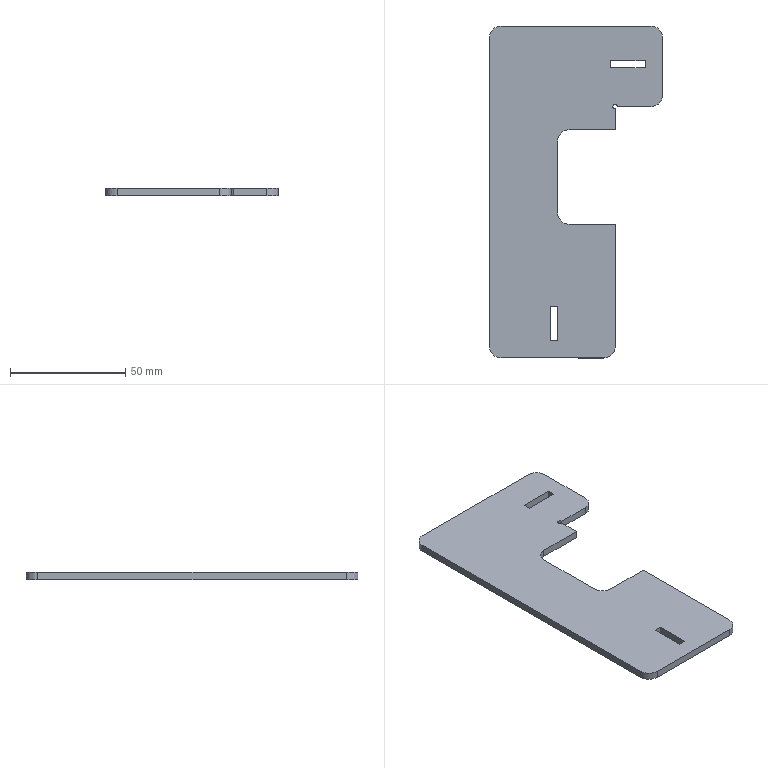Part | SolidWorks | features FlatPattern 1, SMBaseFlange 1, SheetMetal 1 | 1 solid | 29 faces | box 75 x 144 x 3.2 mm | volume 23763 mm3 | plane 20 | cylinder 9 | commonest cylinder face diameters 10 x7 2 x2
STEP:
#1=CARTESIAN_POINT('',(-21.5,109.,3.2));
#2=VERTEX_POINT('',#1);
#3=CARTESIAN_POINT('',(-19.5,109.,3.2));
#4=VERTEX_POINT('',#3);
#5=CARTESIAN_POINT('',(-20.5,109.,3.2));
#6=DIRECTION('',(0.,0.,-1.));
#7=DIRECTION('',(1.,0.,0.));
#8=AXIS2_PLACEMENT_3D('',#5,#6,#7);
#9=CIRCLE('',#8,1.);
#10=EDGE_CURVE('',#2,#4,#9,.T.);
#11=ORIENTED_EDGE('',*,*,#10,.F.);
#12=CARTESIAN_POINT('',(-21.5,109.,0.));
#13=VERTEX_POINT('',#12);
#14=CARTESIAN_POINT('',(-21.5,109.,3.2));
#15=DIRECTION('',(0.,0.,-1.));
#16=VECTOR('',#15,1000.);
#17=LINE('',#14,#16);
#18=EDGE_CURVE('',#2,#13,#17,.T.);
#19=ORIENTED_EDGE('',*,*,#18,.T.);
#20=CARTESIAN_POINT('',(-19.5,109.,0.));
#21=VERTEX_POINT('',#20);
#22=CARTESIAN_POINT('',(-20.5,109.,0.));
#23=DIRECTION('',(0.,0.,-1.));
#24=DIRECTION('',(1.,0.,0.));
#25=AXIS2_PLACEMENT_3D('',#22,#23,#24);
#26=CIRCLE('',#25,1.);
#27=EDGE_CURVE('',#13,#21,#26,.T.);
#28=ORIENTED_EDGE('',*,*,#27,.T.);
#29=CARTESIAN_POINT('',(-19.5,109.,3.2));
#30=DIRECTION('',(0.,0.,-1.));
#31=VECTOR('',#30,1000.);
#32=LINE('',#29,#31);
#33=EDGE_CURVE('',#4,#21,#32,.T.);
#34=ORIENTED_EDGE('',*,*,#33,.F.);
#35=EDGE_LOOP('',(#11,#19,#28,#34));
#36=FACE_OUTER_BOUND('',#35,.T.);
#37=CARTESIAN_POINT('',(-20.5,109.,3.2));
#38=DIRECTION('',(0.,0.,-1.));
#39=DIRECTION('',(-1.,0.,0.));
#40=AXIS2_PLACEMENT_3D('',#37,#38,#39);
#41=CYLINDRICAL_SURFACE('',#40,1.);
#42=ADVANCED_FACE('',(#36),#41,.F.);
#43=CARTESIAN_POINT('',(-7.5,125.8,3.2));
#44=VERTEX_POINT('',#43);
#45=CARTESIAN_POINT('',(-7.5,129.,3.2));
#46=VERTEX_POINT('',#45);
#47=CARTESIAN_POINT('',(-7.5,129.,3.2));
#48=DIRECTION('',(0.,1.,0.));
#49=VECTOR('',#48,1000.);
#50=LINE('',#47,#49);
#51=EDGE_CURVE('',#44,#46,#50,.T.);
#52=ORIENTED_EDGE('',*,*,#51,.F.);
#53=CARTESIAN_POINT('',(-22.5,125.8,3.2));
#54=VERTEX_POINT('',#53);
#55=CARTESIAN_POINT('',(-7.5,125.8,3.2));
#56=DIRECTION('',(1.,0.,0.));
#57=VECTOR('',#56,1000.);
#58=LINE('',#55,#57);
#59=EDGE_CURVE('',#54,#44,#58,.T.);
#60=ORIENTED_EDGE('',*,*,#59,.F.);
#61=CARTESIAN_POINT('',(-22.5,129.,3.2));
#62=VERTEX_POINT('',#61);
#63=CARTESIAN_POINT('',(-22.5,129.,3.2));
#64=DIRECTION('',(0.,-1.,0.));
#65=VECTOR('',#64,1000.);
#66=LINE('',#63,#65);
#67=EDGE_CURVE('',#62,#54,#66,.T.);
#68=ORIENTED_EDGE('',*,*,#67,.F.);
#69=CARTESIAN_POINT('',(-7.5,129.,3.2));
#70=DIRECTION('',(-1.,0.,0.));
#71=VECTOR('',#70,1000.);
#72=LINE('',#69,#71);
#73=EDGE_CURVE('',#46,#62,#72,.T.);
#74=ORIENTED_EDGE('',*,*,#73,.F.);
#75=EDGE_LOOP('',(#52,#60,#68,#74));
#76=FACE_BOUND('',#75,.T.);
#77=CARTESIAN_POINT('',(-40.5,58.,3.2));
#78=VERTEX_POINT('',#77);
#79=CARTESIAN_POINT('',(-45.5,63.,3.2));
#80=VERTEX_POINT('',#79);
#81=CARTESIAN_POINT('',(-40.5,63.,3.2));
#82=DIRECTION('',(0.,0.,-1.));
#83=DIRECTION('',(-1.,0.,0.));
#84=AXIS2_PLACEMENT_3D('',#81,#82,#83);
#85=CIRCLE('',#84,5.);
#86=EDGE_CURVE('',#78,#80,#85,.T.);
#87=ORIENTED_EDGE('',*,*,#86,.T.);
#88=CARTESIAN_POINT('',(-45.5,94.,3.2));
#89=VERTEX_POINT('',#88);
#90=CARTESIAN_POINT('',(-45.5,63.,3.2));
#91=DIRECTION('',(0.,1.,0.));
#92=VECTOR('',#91,1000.);
#93=LINE('',#90,#92);
#94=EDGE_CURVE('',#80,#89,#93,.T.);
#95=ORIENTED_EDGE('',*,*,#94,.T.);
#96=CARTESIAN_POINT('',(-40.5,99.,3.2));
#97=VERTEX_POINT('',#96);
#98=CARTESIAN_POINT('',(-40.5,94.,3.2));
#99=DIRECTION('',(0.,0.,-1.));
#100=DIRECTION('',(-1.,0.,0.));
#101=AXIS2_PLACEMENT_3D('',#98,#99,#100);
#102=CIRCLE('',#101,5.);
#103=EDGE_CURVE('',#89,#97,#102,.T.);
#104=ORIENTED_EDGE('',*,*,#103,.T.);
#105=CARTESIAN_POINT('',(-20.5,99.,3.2));
#106=VERTEX_POINT('',#105);
#107=CARTESIAN_POINT('',(-40.5,99.,3.2));
#108=DIRECTION('',(1.,0.,0.));
#109=VECTOR('',#108,1000.);
#110=LINE('',#107,#109);
#111=EDGE_CURVE('',#97,#106,#110,.T.);
#112=ORIENTED_EDGE('',*,*,#111,.T.);
#113=CARTESIAN_POINT('',(-20.5,108.,3.2));
#114=VERTEX_POINT('',#113);
#115=CARTESIAN_POINT('',(-20.5,99.,3.2));
#116=DIRECTION('',(0.,1.,0.));
#117=VECTOR('',#116,1000.);
#118=LINE('',#115,#117);
#119=EDGE_CURVE('',#106,#114,#118,.T.);
#120=ORIENTED_EDGE('',*,*,#119,.T.);
#121=CARTESIAN_POINT('',(-20.5,109.,3.2));
#122=DIRECTION('',(0.,0.,-1.));
#123=DIRECTION('',(1.,0.,0.));
#124=AXIS2_PLACEMENT_3D('',#121,#122,#123);
#125=CIRCLE('',#124,1.);
#126=EDGE_CURVE('',#114,#2,#125,.T.);
#127=ORIENTED_EDGE('',*,*,#126,.T.);
#128=ORIENTED_EDGE('',*,*,#10,.T.);
#129=CARTESIAN_POINT('',(-5.,109.,3.2));
#130=VERTEX_POINT('',#129);
#131=CARTESIAN_POINT('',(-19.5,109.,3.2));
#132=DIRECTION('',(1.,0.,0.));
#133=VECTOR('',#132,1000.);
#134=LINE('',#131,#133);
#135=EDGE_CURVE('',#4,#130,#134,.T.);
#136=ORIENTED_EDGE('',*,*,#135,.T.);
#137=CARTESIAN_POINT('',(0.,114.,3.2));
#138=VERTEX_POINT('',#137);
#139=CARTESIAN_POINT('',(-5.,114.,3.2));
#140=DIRECTION('',(0.,0.,1.));
#141=DIRECTION('',(1.,0.,0.));
#142=AXIS2_PLACEMENT_3D('',#139,#140,#141);
#143=CIRCLE('',#142,5.);
#144=EDGE_CURVE('',#130,#138,#143,.T.);
#145=ORIENTED_EDGE('',*,*,#144,.T.);
#146=CARTESIAN_POINT('',(0.,139.,3.2));
#147=VERTEX_POINT('',#146);
#148=CARTESIAN_POINT('',(0.,114.,3.2));
#149=DIRECTION('',(0.,1.,0.));
#150=VECTOR('',#149,1000.);
#151=LINE('',#148,#150);
#152=EDGE_CURVE('',#138,#147,#151,.T.);
#153=ORIENTED_EDGE('',*,*,#152,.T.);
#154=CARTESIAN_POINT('',(-5.,144.,3.2));
#155=VERTEX_POINT('',#154);
#156=CARTESIAN_POINT('',(-5.,139.,3.2));
#157=DIRECTION('',(0.,0.,1.));
#158=DIRECTION('',(-1.,0.,0.));
#159=AXIS2_PLACEMENT_3D('',#156,#157,#158);
#160=CIRCLE('',#159,5.);
#161=EDGE_CURVE('',#147,#155,#160,.T.);
#162=ORIENTED_EDGE('',*,*,#161,.T.);
#163=CARTESIAN_POINT('',(-70.,144.,3.2));
#164=VERTEX_POINT('',#163);
#165=CARTESIAN_POINT('',(-5.,144.,3.2));
#166=DIRECTION('',(-1.,0.,0.));
#167=VECTOR('',#166,1000.);
#168=LINE('',#165,#167);
#169=EDGE_CURVE('',#155,#164,#168,.T.);
#170=ORIENTED_EDGE('',*,*,#169,.T.);
#171=CARTESIAN_POINT('',(-75.,139.,3.2));
#172=VERTEX_POINT('',#171);
#173=CARTESIAN_POINT('',(-70.,139.,3.2));
#174=DIRECTION('',(0.,0.,1.));
#175=DIRECTION('',(1.,0.,0.));
#176=AXIS2_PLACEMENT_3D('',#173,#174,#175);
#177=CIRCLE('',#176,5.);
#178=EDGE_CURVE('',#164,#172,#177,.T.);
#179=ORIENTED_EDGE('',*,*,#178,.T.);
#180=CARTESIAN_POINT('',(-75.,5.,3.2));
#181=VERTEX_POINT('',#180);
#182=CARTESIAN_POINT('',(-75.,139.,3.2));
#183=DIRECTION('',(0.,-1.,0.));
#184=VECTOR('',#183,1000.);
#185=LINE('',#182,#184);
#186=EDGE_CURVE('',#172,#181,#185,.T.);
#187=ORIENTED_EDGE('',*,*,#186,.T.);
#188=CARTESIAN_POINT('',(-70.,0.,3.2));
#189=VERTEX_POINT('',#188);
#190=CARTESIAN_POINT('',(-70.,5.,3.2));
#191=DIRECTION('',(0.,0.,1.));
#192=DIRECTION('',(1.,0.,0.));
#193=AXIS2_PLACEMENT_3D('',#190,#191,#192);
#194=CIRCLE('',#193,5.);
#195=EDGE_CURVE('',#181,#189,#194,.T.);
#196=ORIENTED_EDGE('',*,*,#195,.T.);
#197=CARTESIAN_POINT('',(-25.5,0.,3.2));
#198=VERTEX_POINT('',#197);
#199=CARTESIAN_POINT('',(-25.5,0.,3.2));
#200=DIRECTION('',(1.,0.,0.));
#201=VECTOR('',#200,1000.);
#202=LINE('',#199,#201);
#203=EDGE_CURVE('',#189,#198,#202,.T.);
#204=ORIENTED_EDGE('',*,*,#203,.T.);
#205=CARTESIAN_POINT('',(-20.5,5.,3.2));
#206=VERTEX_POINT('',#205);
#207=CARTESIAN_POINT('',(-25.5,5.,3.2));
#208=DIRECTION('',(0.,0.,1.));
#209=DIRECTION('',(-1.,0.,0.));
#210=AXIS2_PLACEMENT_3D('',#207,#208,#209);
#211=CIRCLE('',#210,5.);
#212=EDGE_CURVE('',#198,#206,#211,.T.);
#213=ORIENTED_EDGE('',*,*,#212,.T.);
#214=CARTESIAN_POINT('',(-20.5,58.,3.2));
#215=VERTEX_POINT('',#214);
#216=CARTESIAN_POINT('',(-20.5,58.,3.2));
#217=DIRECTION('',(0.,1.,0.));
#218=VECTOR('',#217,1000.);
#219=LINE('',#216,#218);
#220=EDGE_CURVE('',#206,#215,#219,.T.);
#221=ORIENTED_EDGE('',*,*,#220,.T.);
#222=CARTESIAN_POINT('',(-20.5,58.,3.2));
#223=DIRECTION('',(-1.,0.,0.));
#224=VECTOR('',#223,1000.);
#225=LINE('',#222,#224);
#226=EDGE_CURVE('',#215,#78,#225,.T.);
#227=ORIENTED_EDGE('',*,*,#226,.T.);
#228=EDGE_LOOP('',(#87,#95,#104,#112,#120,#127,#128,#136,#145,#153,#162,#170,#179,#187,#196,#204,#213,#221,#227));
#229=FACE_OUTER_BOUND('',#228,.T.);
#230=CARTESIAN_POINT('',(-45.5,7.5,3.2));
#231=VERTEX_POINT('',#230);
#232=CARTESIAN_POINT('',(-45.5,22.5,3.2));
#233=VERTEX_POINT('',#232);
#234=CARTESIAN_POINT('',(-45.5,7.5,3.2));
#235=DIRECTION('',(0.,1.,0.));
#236=VECTOR('',#235,1000.);
#237=LINE('',#234,#236);
#238=EDGE_CURVE('',#231,#233,#237,.T.);
#239=ORIENTED_EDGE('',*,*,#238,.F.);
#240=CARTESIAN_POINT('',(-48.7,7.5,3.2));
#241=VERTEX_POINT('',#240);
#242=CARTESIAN_POINT('',(-45.5,7.5,3.2));
#243=DIRECTION('',(1.,0.,0.));
#244=VECTOR('',#243,1000.);
#245=LINE('',#242,#244);
#246=EDGE_CURVE('',#241,#231,#245,.T.);
#247=ORIENTED_EDGE('',*,*,#246,.F.);
#248=CARTESIAN_POINT('',(-48.7,22.5,3.2));
#249=VERTEX_POINT('',#248);
#250=CARTESIAN_POINT('',(-48.7,7.5,3.2));
#251=DIRECTION('',(0.,-1.,0.));
#252=VECTOR('',#251,1000.);
#253=LINE('',#250,#252);
#254=EDGE_CURVE('',#249,#241,#253,.T.);
#255=ORIENTED_EDGE('',*,*,#254,.F.);
#256=CARTESIAN_POINT('',(-45.5,22.5,3.2));
#257=DIRECTION('',(-1.,0.,0.));
#258=VECTOR('',#257,1000.);
#259=LINE('',#256,#258);
#260=EDGE_CURVE('',#233,#249,#259,.T.);
#261=ORIENTED_EDGE('',*,*,#260,.F.);
#262=EDGE_LOOP('',(#239,#247,#255,#261));
#263=FACE_BOUND('',#262,.T.);
#264=CARTESIAN_POINT('',(-40.5,63.,3.2));
#265=DIRECTION('',(0.,0.,-1.));
#266=DIRECTION('',(-1.,0.,0.));
#267=AXIS2_PLACEMENT_3D('',#264,#265,#266);
#268=PLANE('',#267);
#269=ADVANCED_FACE('',(#76,#229,#263),#268,.F.);
#270=CARTESIAN_POINT('',(-40.5,58.,0.));
#271=VERTEX_POINT('',#270);
#272=CARTESIAN_POINT('',(-45.5,63.,0.));
#273=VERTEX_POINT('',#272);
#274=CARTESIAN_POINT('',(-40.5,63.,0.));
#275=DIRECTION('',(0.,0.,-1.));
#276=DIRECTION('',(-1.,0.,0.));
#277=AXIS2_PLACEMENT_3D('',#274,#275,#276);
#278=CIRCLE('',#277,5.);
#279=EDGE_CURVE('',#271,#273,#278,.T.);
#280=ORIENTED_EDGE('',*,*,#279,.F.);
#281=CARTESIAN_POINT('',(-20.5,58.,0.));
#282=VERTEX_POINT('',#281);
#283=CARTESIAN_POINT('',(-20.5,58.,0.));
#284=DIRECTION('',(-1.,0.,0.));
#285=VECTOR('',#284,1000.);
#286=LINE('',#283,#285);
#287=EDGE_CURVE('',#282,#271,#286,.T.);
#288=ORIENTED_EDGE('',*,*,#287,.F.);
#289=CARTESIAN_POINT('',(-20.5,5.,0.));
#290=VERTEX_POINT('',#289);
#291=CARTESIAN_POINT('',(-20.5,58.,0.));
#292=DIRECTION('',(0.,1.,0.));
#293=VECTOR('',#292,1000.);
#294=LINE('',#291,#293);
#295=EDGE_CURVE('',#290,#282,#294,.T.);
#296=ORIENTED_EDGE('',*,*,#295,.F.);
#297=CARTESIAN_POINT('',(-25.5,0.,0.));
#298=VERTEX_POINT('',#297);
#299=CARTESIAN_POINT('',(-25.5,5.,0.));
#300=DIRECTION('',(0.,0.,1.));
#301=DIRECTION('',(-1.,0.,0.));
#302=AXIS2_PLACEMENT_3D('',#299,#300,#301);
#303=CIRCLE('',#302,5.);
#304=EDGE_CURVE('',#298,#290,#303,.T.);
#305=ORIENTED_EDGE('',*,*,#304,.F.);
#306=CARTESIAN_POINT('',(-70.,0.,0.));
#307=VERTEX_POINT('',#306);
#308=CARTESIAN_POINT('',(-25.5,0.,0.));
#309=DIRECTION('',(1.,0.,0.));
#310=VECTOR('',#309,1000.);
#311=LINE('',#308,#310);
#312=EDGE_CURVE('',#307,#298,#311,.T.);
#313=ORIENTED_EDGE('',*,*,#312,.F.);
#314=CARTESIAN_POINT('',(-75.,5.,0.));
#315=VERTEX_POINT('',#314);
#316=CARTESIAN_POINT('',(-70.,5.,0.));
#317=DIRECTION('',(0.,0.,1.));
#318=DIRECTION('',(1.,0.,0.));
#319=AXIS2_PLACEMENT_3D('',#316,#317,#318);
#320=CIRCLE('',#319,5.);
#321=EDGE_CURVE('',#315,#307,#320,.T.);
#322=ORIENTED_EDGE('',*,*,#321,.F.);
#323=CARTESIAN_POINT('',(-75.,139.,0.));
#324=VERTEX_POINT('',#323);
#325=CARTESIAN_POINT('',(-75.,139.,0.));
#326=DIRECTION('',(0.,-1.,0.));
#327=VECTOR('',#326,1000.);
#328=LINE('',#325,#327);
#329=EDGE_CURVE('',#324,#315,#328,.T.);
#330=ORIENTED_EDGE('',*,*,#329,.F.);
#331=CARTESIAN_POINT('',(-70.,144.,0.));
#332=VERTEX_POINT('',#331);
#333=CARTESIAN_POINT('',(-70.,139.,0.));
#334=DIRECTION('',(0.,0.,1.));
#335=DIRECTION('',(1.,0.,0.));
#336=AXIS2_PLACEMENT_3D('',#333,#334,#335);
#337=CIRCLE('',#336,5.);
#338=EDGE_CURVE('',#332,#324,#337,.T.);
#339=ORIENTED_EDGE('',*,*,#338,.F.);
#340=CARTESIAN_POINT('',(-5.,144.,0.));
#341=VERTEX_POINT('',#340);
#342=CARTESIAN_POINT('',(-5.,144.,0.));
#343=DIRECTION('',(-1.,0.,0.));
#344=VECTOR('',#343,1000.);
#345=LINE('',#342,#344);
#346=EDGE_CURVE('',#341,#332,#345,.T.);
#347=ORIENTED_EDGE('',*,*,#346,.F.);
#348=CARTESIAN_POINT('',(0.,139.,0.));
#349=VERTEX_POINT('',#348);
#350=CARTESIAN_POINT('',(-5.,139.,0.));
#351=DIRECTION('',(0.,0.,1.));
#352=DIRECTION('',(-1.,0.,0.));
#353=AXIS2_PLACEMENT_3D('',#350,#351,#352);
#354=CIRCLE('',#353,5.);
#355=EDGE_CURVE('',#349,#341,#354,.T.);
#356=ORIENTED_EDGE('',*,*,#355,.F.);
#357=CARTESIAN_POINT('',(0.,114.,0.));
#358=VERTEX_POINT('',#357);
#359=CARTESIAN_POINT('',(0.,114.,0.));
#360=DIRECTION('',(0.,1.,0.));
#361=VECTOR('',#360,1000.);
#362=LINE('',#359,#361);
#363=EDGE_CURVE('',#358,#349,#362,.T.);
#364=ORIENTED_EDGE('',*,*,#363,.F.);
#365=CARTESIAN_POINT('',(-5.,109.,0.));
#366=VERTEX_POINT('',#365);
#367=CARTESIAN_POINT('',(-5.,114.,0.));
#368=DIRECTION('',(0.,0.,1.));
#369=DIRECTION('',(1.,0.,0.));
#370=AXIS2_PLACEMENT_3D('',#367,#368,#369);
#371=CIRCLE('',#370,5.);
#372=EDGE_CURVE('',#366,#358,#371,.T.);
#373=ORIENTED_EDGE('',*,*,#372,.F.);
#374=CARTESIAN_POINT('',(-19.5,109.,0.));
#375=DIRECTION('',(1.,0.,0.));
#376=VECTOR('',#375,1000.);
#377=LINE('',#374,#376);
#378=EDGE_CURVE('',#21,#366,#377,.T.);
#379=ORIENTED_EDGE('',*,*,#378,.F.);
#380=ORIENTED_EDGE('',*,*,#27,.F.);
#381=CARTESIAN_POINT('',(-20.5,108.,0.));
#382=VERTEX_POINT('',#381);
#383=CARTESIAN_POINT('',(-20.5,109.,0.));
#384=DIRECTION('',(0.,0.,-1.));
#385=DIRECTION('',(1.,0.,0.));
#386=AXIS2_PLACEMENT_3D('',#383,#384,#385);
#387=CIRCLE('',#386,1.);
#388=EDGE_CURVE('',#382,#13,#387,.T.);
#389=ORIENTED_EDGE('',*,*,#388,.F.);
#390=CARTESIAN_POINT('',(-20.5,99.,0.));
#391=VERTEX_POINT('',#390);
#392=CARTESIAN_POINT('',(-20.5,99.,0.));
#393=DIRECTION('',(0.,1.,0.));
#394=VECTOR('',#393,1000.);
#395=LINE('',#392,#394);
#396=EDGE_CURVE('',#391,#382,#395,.T.);
#397=ORIENTED_EDGE('',*,*,#396,.F.);
#398=CARTESIAN_POINT('',(-40.5,99.,0.));
#399=VERTEX_POINT('',#398);
#400=CARTESIAN_POINT('',(-40.5,99.,0.));
#401=DIRECTION('',(1.,0.,0.));
#402=VECTOR('',#401,1000.);
#403=LINE('',#400,#402);
#404=EDGE_CURVE('',#399,#391,#403,.T.);
#405=ORIENTED_EDGE('',*,*,#404,.F.);
#406=CARTESIAN_POINT('',(-45.5,94.,0.));
#407=VERTEX_POINT('',#406);
#408=CARTESIAN_POINT('',(-40.5,94.,0.));
#409=DIRECTION('',(0.,0.,-1.));
#410=DIRECTION('',(-1.,0.,0.));
#411=AXIS2_PLACEMENT_3D('',#408,#409,#410);
#412=CIRCLE('',#411,5.);
#413=EDGE_CURVE('',#407,#399,#412,.T.);
#414=ORIENTED_EDGE('',*,*,#413,.F.);
#415=CARTESIAN_POINT('',(-45.5,63.,0.));
#416=DIRECTION('',(0.,1.,0.));
#417=VECTOR('',#416,1000.);
#418=LINE('',#415,#417);
#419=EDGE_CURVE('',#273,#407,#418,.T.);
#420=ORIENTED_EDGE('',*,*,#419,.F.);
#421=EDGE_LOOP('',(#280,#288,#296,#305,#313,#322,#330,#339,#347,#356,#364,#373,#379,#380,#389,#397,#405,#414,#420));
#422=FACE_OUTER_BOUND('',#421,.T.);
#423=CARTESIAN_POINT('',(-22.5,125.8,0.));
#424=VERTEX_POINT('',#423);
#425=CARTESIAN_POINT('',(-7.5,125.8,0.));
#426=VERTEX_POINT('',#425);
#427=CARTESIAN_POINT('',(-7.5,125.8,0.));
#428=DIRECTION('',(1.,0.,0.));
#429=VECTOR('',#428,1000.);
#430=LINE('',#427,#429);
#431=EDGE_CURVE('',#424,#426,#430,.T.);
#432=ORIENTED_EDGE('',*,*,#431,.T.);
#433=CARTESIAN_POINT('',(-7.5,129.,0.));
#434=VERTEX_POINT('',#433);
#435=CARTESIAN_POINT('',(-7.5,129.,0.));
#436=DIRECTION('',(0.,1.,0.));
#437=VECTOR('',#436,1000.);
#438=LINE('',#435,#437);
#439=EDGE_CURVE('',#426,#434,#438,.T.);
#440=ORIENTED_EDGE('',*,*,#439,.T.);
#441=CARTESIAN_POINT('',(-22.5,129.,0.));
#442=VERTEX_POINT('',#441);
#443=CARTESIAN_POINT('',(-7.5,129.,0.));
#444=DIRECTION('',(-1.,0.,0.));
#445=VECTOR('',#444,1000.);
#446=LINE('',#443,#445);
#447=EDGE_CURVE('',#434,#442,#446,.T.);
#448=ORIENTED_EDGE('',*,*,#447,.T.);
#449=CARTESIAN_POINT('',(-22.5,129.,0.));
#450=DIRECTION('',(0.,-1.,0.));
#451=VECTOR('',#450,1000.);
#452=LINE('',#449,#451);
#453=EDGE_CURVE('',#442,#424,#452,.T.);
#454=ORIENTED_EDGE('',*,*,#453,.T.);
#455=EDGE_LOOP('',(#432,#440,#448,#454));
#456=FACE_BOUND('',#455,.T.);
#457=CARTESIAN_POINT('',(-48.7,7.5,0.));
#458=VERTEX_POINT('',#457);
#459=CARTESIAN_POINT('',(-45.5,7.5,0.));
#460=VERTEX_POINT('',#459);
#461=CARTESIAN_POINT('',(-45.5,7.5,0.));
#462=DIRECTION('',(1.,0.,0.));
#463=VECTOR('',#462,1000.);
#464=LINE('',#461,#463);
#465=EDGE_CURVE('',#458,#460,#464,.T.);
#466=ORIENTED_EDGE('',*,*,#465,.T.);
#467=CARTESIAN_POINT('',(-45.5,22.5,0.));
#468=VERTEX_POINT('',#467);
#469=CARTESIAN_POINT('',(-45.5,7.5,0.));
#470=DIRECTION('',(0.,1.,0.));
#471=VECTOR('',#470,1000.);
#472=LINE('',#469,#471);
#473=EDGE_CURVE('',#460,#468,#472,.T.);
#474=ORIENTED_EDGE('',*,*,#473,.T.);
#475=CARTESIAN_POINT('',(-48.7,22.5,0.));
#476=VERTEX_POINT('',#475);
#477=CARTESIAN_POINT('',(-45.5,22.5,0.));
#478=DIRECTION('',(-1.,0.,0.));
#479=VECTOR('',#478,1000.);
#480=LINE('',#477,#479);
#481=EDGE_CURVE('',#468,#476,#480,.T.);
#482=ORIENTED_EDGE('',*,*,#481,.T.);
#483=CARTESIAN_POINT('',(-48.7,7.5,0.));
#484=DIRECTION('',(0.,-1.,0.));
#485=VECTOR('',#484,1000.);
#486=LINE('',#483,#485);
#487=EDGE_CURVE('',#476,#458,#486,.T.);
#488=ORIENTED_EDGE('',*,*,#487,.T.);
#489=EDGE_LOOP('',(#466,#474,#482,#488));
#490=FACE_BOUND('',#489,.T.);
#491=CARTESIAN_POINT('',(-40.5,63.,0.));
#492=DIRECTION('',(0.,0.,-1.));
#493=DIRECTION('',(-1.,0.,0.));
#494=AXIS2_PLACEMENT_3D('',#491,#492,#493);
#495=PLANE('',#494);
#496=ADVANCED_FACE('',(#422,#456,#490),#495,.T.);
#497=ORIENTED_EDGE('',*,*,#279,.T.);
#498=CARTESIAN_POINT('',(-45.5,63.,3.2));
#499=DIRECTION('',(0.,0.,-1.));
#500=VECTOR('',#499,1000.);
#501=LINE('',#498,#500);
#502=EDGE_CURVE('',#80,#273,#501,.T.);
#503=ORIENTED_EDGE('',*,*,#502,.F.);
#504=ORIENTED_EDGE('',*,*,#86,.F.);
#505=CARTESIAN_POINT('',(-40.5,58.,3.2));
#506=DIRECTION('',(0.,0.,-1.));
#507=VECTOR('',#506,1000.);
#508=LINE('',#505,#507);
#509=EDGE_CURVE('',#78,#271,#508,.T.);
#510=ORIENTED_EDGE('',*,*,#509,.T.);
#511=EDGE_LOOP('',(#497,#503,#504,#510));
#512=FACE_OUTER_BOUND('',#511,.T.);
#513=CARTESIAN_POINT('',(-40.5,63.,3.2));
#514=DIRECTION('',(0.,0.,-1.));
#515=DIRECTION('',(-1.,0.,0.));
#516=AXIS2_PLACEMENT_3D('',#513,#514,#515);
#517=CYLINDRICAL_SURFACE('',#516,5.);
#518=ADVANCED_FACE('',(#512),#517,.F.);
#519=ORIENTED_EDGE('',*,*,#419,.T.);
#520=CARTESIAN_POINT('',(-45.5,94.,3.2));
#521=DIRECTION('',(0.,0.,-1.));
#522=VECTOR('',#521,1000.);
#523=LINE('',#520,#522);
#524=EDGE_CURVE('',#89,#407,#523,.T.);
#525=ORIENTED_EDGE('',*,*,#524,.F.);
#526=ORIENTED_EDGE('',*,*,#94,.F.);
#527=ORIENTED_EDGE('',*,*,#502,.T.);
#528=EDGE_LOOP('',(#519,#525,#526,#527));
#529=FACE_OUTER_BOUND('',#528,.T.);
#530=CARTESIAN_POINT('',(-45.5,63.,3.2));
#531=DIRECTION('',(-1.,0.,0.));
#532=DIRECTION('',(0.,0.,1.));
#533=AXIS2_PLACEMENT_3D('',#530,#531,#532);
#534=PLANE('',#533);
#535=ADVANCED_FACE('',(#529),#534,.F.);
#536=ORIENTED_EDGE('',*,*,#413,.T.);
#537=CARTESIAN_POINT('',(-40.5,99.,3.2));
#538=DIRECTION('',(0.,0.,-1.));
#539=VECTOR('',#538,1000.);
#540=LINE('',#537,#539);
#541=EDGE_CURVE('',#97,#399,#540,.T.);
#542=ORIENTED_EDGE('',*,*,#541,.F.);
#543=ORIENTED_EDGE('',*,*,#103,.F.);
#544=ORIENTED_EDGE('',*,*,#524,.T.);
#545=EDGE_LOOP('',(#536,#542,#543,#544));
#546=FACE_OUTER_BOUND('',#545,.T.);
#547=CARTESIAN_POINT('',(-40.5,94.,3.2));
#548=DIRECTION('',(0.,0.,-1.));
#549=DIRECTION('',(-1.,0.,0.));
#550=AXIS2_PLACEMENT_3D('',#547,#548,#549);
#551=CYLINDRICAL_SURFACE('',#550,5.);
#552=ADVANCED_FACE('',(#546),#551,.F.);
#553=ORIENTED_EDGE('',*,*,#404,.T.);
#554=CARTESIAN_POINT('',(-20.5,99.,3.2));
#555=DIRECTION('',(0.,0.,-1.));
#556=VECTOR('',#555,1000.);
#557=LINE('',#554,#556);
#558=EDGE_CURVE('',#106,#391,#557,.T.);
#559=ORIENTED_EDGE('',*,*,#558,.F.);
#560=ORIENTED_EDGE('',*,*,#111,.F.);
#561=ORIENTED_EDGE('',*,*,#541,.T.);
#562=EDGE_LOOP('',(#553,#559,#560,#561));
#563=FACE_OUTER_BOUND('',#562,.T.);
#564=CARTESIAN_POINT('',(-40.5,99.,3.2));
#565=DIRECTION('',(0.,1.,0.));
#566=DIRECTION('',(0.,0.,1.));
#567=AXIS2_PLACEMENT_3D('',#564,#565,#566);
#568=PLANE('',#567);
#569=ADVANCED_FACE('',(#563),#568,.F.);
#570=ORIENTED_EDGE('',*,*,#396,.T.);
#571=CARTESIAN_POINT('',(-20.5,108.,3.2));
#572=DIRECTION('',(0.,0.,-1.));
#573=VECTOR('',#572,1000.);
#574=LINE('',#571,#573);
#575=EDGE_CURVE('',#114,#382,#574,.T.);
#576=ORIENTED_EDGE('',*,*,#575,.F.);
#577=ORIENTED_EDGE('',*,*,#119,.F.);
#578=ORIENTED_EDGE('',*,*,#558,.T.);
#579=EDGE_LOOP('',(#570,#576,#577,#578));
#580=FACE_OUTER_BOUND('',#579,.T.);
#581=CARTESIAN_POINT('',(-20.5,99.,3.2));
#582=DIRECTION('',(-1.,0.,0.));
#583=DIRECTION('',(0.,-1.,0.));
#584=AXIS2_PLACEMENT_3D('',#581,#582,#583);
#585=PLANE('',#584);
#586=ADVANCED_FACE('',(#580),#585,.F.);
#587=ORIENTED_EDGE('',*,*,#18,.F.);
#588=ORIENTED_EDGE('',*,*,#126,.F.);
#589=ORIENTED_EDGE('',*,*,#575,.T.);
#590=ORIENTED_EDGE('',*,*,#388,.T.);
#591=EDGE_LOOP('',(#587,#588,#589,#590));
#592=FACE_OUTER_BOUND('',#591,.T.);
#593=CARTESIAN_POINT('',(-20.5,109.,3.2));
#594=DIRECTION('',(0.,0.,-1.));
#595=DIRECTION('',(-1.,0.,0.));
#596=AXIS2_PLACEMENT_3D('',#593,#594,#595);
#597=CYLINDRICAL_SURFACE('',#596,1.);
#598=ADVANCED_FACE('',(#592),#597,.F.);
#599=ORIENTED_EDGE('',*,*,#378,.T.);
#600=CARTESIAN_POINT('',(-5.,109.,3.2));
#601=DIRECTION('',(0.,0.,-1.));
#602=VECTOR('',#601,1000.);
#603=LINE('',#600,#602);
#604=EDGE_CURVE('',#130,#366,#603,.T.);
#605=ORIENTED_EDGE('',*,*,#604,.F.);
#606=ORIENTED_EDGE('',*,*,#135,.F.);
#607=ORIENTED_EDGE('',*,*,#33,.T.);
#608=EDGE_LOOP('',(#599,#605,#606,#607));
#609=FACE_OUTER_BOUND('',#608,.T.);
#610=CARTESIAN_POINT('',(-19.5,109.,3.2));
#611=DIRECTION('',(0.,1.,0.));
#612=DIRECTION('',(-1.,0.,0.));
#613=AXIS2_PLACEMENT_3D('',#610,#611,#612);
#614=PLANE('',#613);
#615=ADVANCED_FACE('',(#609),#614,.F.);
#616=ORIENTED_EDGE('',*,*,#372,.T.);
#617=CARTESIAN_POINT('',(0.,114.,3.2));
#618=DIRECTION('',(0.,0.,-1.));
#619=VECTOR('',#618,1000.);
#620=LINE('',#617,#619);
#621=EDGE_CURVE('',#138,#358,#620,.T.);
#622=ORIENTED_EDGE('',*,*,#621,.F.);
#623=ORIENTED_EDGE('',*,*,#144,.F.);
#624=ORIENTED_EDGE('',*,*,#604,.T.);
#625=EDGE_LOOP('',(#616,#622,#623,#624));
#626=FACE_OUTER_BOUND('',#625,.T.);
#627=CARTESIAN_POINT('',(-5.,114.,3.2));
#628=DIRECTION('',(0.,0.,-1.));
#629=DIRECTION('',(-1.,0.,0.));
#630=AXIS2_PLACEMENT_3D('',#627,#628,#629);
#631=CYLINDRICAL_SURFACE('',#630,5.);
#632=ADVANCED_FACE('',(#626),#631,.T.);
#633=ORIENTED_EDGE('',*,*,#363,.T.);
#634=CARTESIAN_POINT('',(0.,139.,3.2));
#635=DIRECTION('',(0.,0.,-1.));
#636=VECTOR('',#635,1000.);
#637=LINE('',#634,#636);
#638=EDGE_CURVE('',#147,#349,#637,.T.);
#639=ORIENTED_EDGE('',*,*,#638,.F.);
#640=ORIENTED_EDGE('',*,*,#152,.F.);
#641=ORIENTED_EDGE('',*,*,#621,.T.);
#642=EDGE_LOOP('',(#633,#639,#640,#641));
#643=FACE_OUTER_BOUND('',#642,.T.);
#644=CARTESIAN_POINT('',(0.,114.,3.2));
#645=DIRECTION('',(-1.,0.,0.));
#646=DIRECTION('',(0.,-1.,0.));
#647=AXIS2_PLACEMENT_3D('',#644,#645,#646);
#648=PLANE('',#647);
#649=ADVANCED_FACE('',(#643),#648,.F.);
#650=ORIENTED_EDGE('',*,*,#355,.T.);
#651=CARTESIAN_POINT('',(-5.,144.,3.2));
#652=DIRECTION('',(0.,0.,-1.));
#653=VECTOR('',#652,1000.);
#654=LINE('',#651,#653);
#655=EDGE_CURVE('',#155,#341,#654,.T.);
#656=ORIENTED_EDGE('',*,*,#655,.F.);
#657=ORIENTED_EDGE('',*,*,#161,.F.);
#658=ORIENTED_EDGE('',*,*,#638,.T.);
#659=EDGE_LOOP('',(#650,#656,#657,#658));
#660=FACE_OUTER_BOUND('',#659,.T.);
#661=CARTESIAN_POINT('',(-5.,139.,3.2));
#662=DIRECTION('',(0.,0.,-1.));
#663=DIRECTION('',(-1.,0.,0.));
#664=AXIS2_PLACEMENT_3D('',#661,#662,#663);
#665=CYLINDRICAL_SURFACE('',#664,5.);
#666=ADVANCED_FACE('',(#660),#665,.T.);
#667=ORIENTED_EDGE('',*,*,#346,.T.);
#668=CARTESIAN_POINT('',(-70.,144.,3.2));
#669=DIRECTION('',(0.,0.,-1.));
#670=VECTOR('',#669,1000.);
#671=LINE('',#668,#670);
#672=EDGE_CURVE('',#164,#332,#671,.T.);
#673=ORIENTED_EDGE('',*,*,#672,.F.);
#674=ORIENTED_EDGE('',*,*,#169,.F.);
#675=ORIENTED_EDGE('',*,*,#655,.T.);
#676=EDGE_LOOP('',(#667,#673,#674,#675));
#677=FACE_OUTER_BOUND('',#676,.T.);
#678=CARTESIAN_POINT('',(-5.,144.,3.2));
#679=DIRECTION('',(0.,-1.,0.));
#680=DIRECTION('',(0.,0.,-1.));
#681=AXIS2_PLACEMENT_3D('',#678,#679,#680);
#682=PLANE('',#681);
#683=ADVANCED_FACE('',(#677),#682,.F.);
#684=ORIENTED_EDGE('',*,*,#338,.T.);
#685=CARTESIAN_POINT('',(-75.,139.,3.2));
#686=DIRECTION('',(0.,0.,-1.));
#687=VECTOR('',#686,1000.);
#688=LINE('',#685,#687);
#689=EDGE_CURVE('',#172,#324,#688,.T.);
#690=ORIENTED_EDGE('',*,*,#689,.F.);
#691=ORIENTED_EDGE('',*,*,#178,.F.);
#692=ORIENTED_EDGE('',*,*,#672,.T.);
#693=EDGE_LOOP('',(#684,#690,#691,#692));
#694=FACE_OUTER_BOUND('',#693,.T.);
#695=CARTESIAN_POINT('',(-70.,139.,3.2));
#696=DIRECTION('',(0.,0.,-1.));
#697=DIRECTION('',(-1.,0.,0.));
#698=AXIS2_PLACEMENT_3D('',#695,#696,#697);
#699=CYLINDRICAL_SURFACE('',#698,5.);
#700=ADVANCED_FACE('',(#694),#699,.T.);
#701=ORIENTED_EDGE('',*,*,#329,.T.);
#702=CARTESIAN_POINT('',(-75.,5.,3.2));
#703=DIRECTION('',(0.,0.,-1.));
#704=VECTOR('',#703,1000.);
#705=LINE('',#702,#704);
#706=EDGE_CURVE('',#181,#315,#705,.T.);
#707=ORIENTED_EDGE('',*,*,#706,.F.);
#708=ORIENTED_EDGE('',*,*,#186,.F.);
#709=ORIENTED_EDGE('',*,*,#689,.T.);
#710=EDGE_LOOP('',(#701,#707,#708,#709));
#711=FACE_OUTER_BOUND('',#710,.T.);
#712=CARTESIAN_POINT('',(-75.,139.,3.2));
#713=DIRECTION('',(1.,0.,0.));
#714=DIRECTION('',(0.,1.,0.));
#715=AXIS2_PLACEMENT_3D('',#712,#713,#714);
#716=PLANE('',#715);
#717=ADVANCED_FACE('',(#711),#716,.F.);
#718=ORIENTED_EDGE('',*,*,#321,.T.);
#719=CARTESIAN_POINT('',(-70.,0.,3.2));
#720=DIRECTION('',(0.,0.,-1.));
#721=VECTOR('',#720,1000.);
#722=LINE('',#719,#721);
#723=EDGE_CURVE('',#189,#307,#722,.T.);
#724=ORIENTED_EDGE('',*,*,#723,.F.);
#725=ORIENTED_EDGE('',*,*,#195,.F.);
#726=ORIENTED_EDGE('',*,*,#706,.T.);
#727=EDGE_LOOP('',(#718,#724,#725,#726));
#728=FACE_OUTER_BOUND('',#727,.T.);
#729=CARTESIAN_POINT('',(-70.,5.,3.2));
#730=DIRECTION('',(0.,0.,-1.));
#731=DIRECTION('',(-1.,0.,0.));
#732=AXIS2_PLACEMENT_3D('',#729,#730,#731);
#733=CYLINDRICAL_SURFACE('',#732,5.);
#734=ADVANCED_FACE('',(#728),#733,.T.);
#735=ORIENTED_EDGE('',*,*,#312,.T.);
#736=CARTESIAN_POINT('',(-25.5,0.,3.2));
#737=DIRECTION('',(0.,0.,-1.));
#738=VECTOR('',#737,1000.);
#739=LINE('',#736,#738);
#740=EDGE_CURVE('',#198,#298,#739,.T.);
#741=ORIENTED_EDGE('',*,*,#740,.F.);
#742=ORIENTED_EDGE('',*,*,#203,.F.);
#743=ORIENTED_EDGE('',*,*,#723,.T.);
#744=EDGE_LOOP('',(#735,#741,#742,#743));
#745=FACE_OUTER_BOUND('',#744,.T.);
#746=CARTESIAN_POINT('',(-25.5,0.,3.2));
#747=DIRECTION('',(0.,1.,0.));
#748=DIRECTION('',(-1.,0.,0.));
#749=AXIS2_PLACEMENT_3D('',#746,#747,#748);
#750=PLANE('',#749);
#751=ADVANCED_FACE('',(#745),#750,.F.);
#752=ORIENTED_EDGE('',*,*,#304,.T.);
#753=CARTESIAN_POINT('',(-20.5,5.,3.2));
#754=DIRECTION('',(0.,0.,-1.));
#755=VECTOR('',#754,1000.);
#756=LINE('',#753,#755);
#757=EDGE_CURVE('',#206,#290,#756,.T.);
#758=ORIENTED_EDGE('',*,*,#757,.F.);
#759=ORIENTED_EDGE('',*,*,#212,.F.);
#760=ORIENTED_EDGE('',*,*,#740,.T.);
#761=EDGE_LOOP('',(#752,#758,#759,#760));
#762=FACE_OUTER_BOUND('',#761,.T.);
#763=CARTESIAN_POINT('',(-25.5,5.,3.2));
#764=DIRECTION('',(0.,0.,-1.));
#765=DIRECTION('',(-1.,0.,0.));
#766=AXIS2_PLACEMENT_3D('',#763,#764,#765);
#767=CYLINDRICAL_SURFACE('',#766,5.);
#768=ADVANCED_FACE('',(#762),#767,.T.);
#769=ORIENTED_EDGE('',*,*,#295,.T.);
#770=CARTESIAN_POINT('',(-20.5,58.,3.2));
#771=DIRECTION('',(0.,0.,-1.));
#772=VECTOR('',#771,1000.);
#773=LINE('',#770,#772);
#774=EDGE_CURVE('',#215,#282,#773,.T.);
#775=ORIENTED_EDGE('',*,*,#774,.F.);
#776=ORIENTED_EDGE('',*,*,#220,.F.);
#777=ORIENTED_EDGE('',*,*,#757,.T.);
#778=EDGE_LOOP('',(#769,#775,#776,#777));
#779=FACE_OUTER_BOUND('',#778,.T.);
#780=CARTESIAN_POINT('',(-20.5,58.,3.2));
#781=DIRECTION('',(-1.,0.,0.));
#782=DIRECTION('',(0.,0.,1.));
#783=AXIS2_PLACEMENT_3D('',#780,#781,#782);
#784=PLANE('',#783);
#785=ADVANCED_FACE('',(#779),#784,.F.);
#786=ORIENTED_EDGE('',*,*,#287,.T.);
#787=ORIENTED_EDGE('',*,*,#509,.F.);
#788=ORIENTED_EDGE('',*,*,#226,.F.);
#789=ORIENTED_EDGE('',*,*,#774,.T.);
#790=EDGE_LOOP('',(#786,#787,#788,#789));
#791=FACE_OUTER_BOUND('',#790,.T.);
#792=CARTESIAN_POINT('',(-20.5,58.,3.2));
#793=DIRECTION('',(0.,-1.,0.));
#794=DIRECTION('',(0.,0.,-1.));
#795=AXIS2_PLACEMENT_3D('',#792,#793,#794);
#796=PLANE('',#795);
#797=ADVANCED_FACE('',(#791),#796,.F.);
#798=ORIENTED_EDGE('',*,*,#439,.F.);
#799=CARTESIAN_POINT('',(-7.5,125.8,3.2));
#800=DIRECTION('',(0.,0.,-1.));
#801=VECTOR('',#800,1000.);
#802=LINE('',#799,#801);
#803=EDGE_CURVE('',#44,#426,#802,.T.);
#804=ORIENTED_EDGE('',*,*,#803,.F.);
#805=ORIENTED_EDGE('',*,*,#51,.T.);
#806=CARTESIAN_POINT('',(-7.5,129.,3.2));
#807=DIRECTION('',(0.,0.,-1.));
#808=VECTOR('',#807,1000.);
#809=LINE('',#806,#808);
#810=EDGE_CURVE('',#46,#434,#809,.T.);
#811=ORIENTED_EDGE('',*,*,#810,.T.);
#812=EDGE_LOOP('',(#798,#804,#805,#811));
#813=FACE_OUTER_BOUND('',#812,.T.);
#814=CARTESIAN_POINT('',(-7.5,129.,3.2));
#815=DIRECTION('',(-1.,0.,0.));
#816=DIRECTION('',(0.,0.,1.));
#817=AXIS2_PLACEMENT_3D('',#814,#815,#816);
#818=PLANE('',#817);
#819=ADVANCED_FACE('',(#813),#818,.T.);
#820=ORIENTED_EDGE('',*,*,#447,.F.);
#821=ORIENTED_EDGE('',*,*,#810,.F.);
#822=ORIENTED_EDGE('',*,*,#73,.T.);
#823=CARTESIAN_POINT('',(-22.5,129.,3.2));
#824=DIRECTION('',(0.,0.,-1.));
#825=VECTOR('',#824,1000.);
#826=LINE('',#823,#825);
#827=EDGE_CURVE('',#62,#442,#826,.T.);
#828=ORIENTED_EDGE('',*,*,#827,.T.);
#829=EDGE_LOOP('',(#820,#821,#822,#828));
#830=FACE_OUTER_BOUND('',#829,.T.);
#831=CARTESIAN_POINT('',(-7.5,129.,3.2));
#832=DIRECTION('',(0.,-1.,0.));
#833=DIRECTION('',(0.,0.,-1.));
#834=AXIS2_PLACEMENT_3D('',#831,#832,#833);
#835=PLANE('',#834);
#836=ADVANCED_FACE('',(#830),#835,.T.);
#837=ORIENTED_EDGE('',*,*,#453,.F.);
#838=ORIENTED_EDGE('',*,*,#827,.F.);
#839=ORIENTED_EDGE('',*,*,#67,.T.);
#840=CARTESIAN_POINT('',(-22.5,125.8,3.2));
#841=DIRECTION('',(0.,0.,-1.));
#842=VECTOR('',#841,1000.);
#843=LINE('',#840,#842);
#844=EDGE_CURVE('',#54,#424,#843,.T.);
#845=ORIENTED_EDGE('',*,*,#844,.T.);
#846=EDGE_LOOP('',(#837,#838,#839,#845));
#847=FACE_OUTER_BOUND('',#846,.T.);
#848=CARTESIAN_POINT('',(-22.5,129.,3.2));
#849=DIRECTION('',(1.,0.,0.));
#850=DIRECTION('',(0.,0.,-1.));
#851=AXIS2_PLACEMENT_3D('',#848,#849,#850);
#852=PLANE('',#851);
#853=ADVANCED_FACE('',(#847),#852,.T.);
#854=ORIENTED_EDGE('',*,*,#431,.F.);
#855=ORIENTED_EDGE('',*,*,#844,.F.);
#856=ORIENTED_EDGE('',*,*,#59,.T.);
#857=ORIENTED_EDGE('',*,*,#803,.T.);
#858=EDGE_LOOP('',(#854,#855,#856,#857));
#859=FACE_OUTER_BOUND('',#858,.T.);
#860=CARTESIAN_POINT('',(-7.5,125.8,3.2));
#861=DIRECTION('',(0.,1.,0.));
#862=DIRECTION('',(0.,0.,1.));
#863=AXIS2_PLACEMENT_3D('',#860,#861,#862);
#864=PLANE('',#863);
#865=ADVANCED_FACE('',(#859),#864,.T.);
#866=ORIENTED_EDGE('',*,*,#473,.F.);
#867=CARTESIAN_POINT('',(-45.5,7.5,3.2));
#868=DIRECTION('',(0.,0.,-1.));
#869=VECTOR('',#868,1000.);
#870=LINE('',#867,#869);
#871=EDGE_CURVE('',#231,#460,#870,.T.);
#872=ORIENTED_EDGE('',*,*,#871,.F.);
#873=ORIENTED_EDGE('',*,*,#238,.T.);
#874=CARTESIAN_POINT('',(-45.5,22.5,3.2));
#875=DIRECTION('',(0.,0.,-1.));
#876=VECTOR('',#875,1000.);
#877=LINE('',#874,#876);
#878=EDGE_CURVE('',#233,#468,#877,.T.);
#879=ORIENTED_EDGE('',*,*,#878,.T.);
#880=EDGE_LOOP('',(#866,#872,#873,#879));
#881=FACE_OUTER_BOUND('',#880,.T.);
#882=CARTESIAN_POINT('',(-45.5,7.5,3.2));
#883=DIRECTION('',(-1.,0.,0.));
#884=DIRECTION('',(0.,0.,1.));
#885=AXIS2_PLACEMENT_3D('',#882,#883,#884);
#886=PLANE('',#885);
#887=ADVANCED_FACE('',(#881),#886,.T.);
#888=ORIENTED_EDGE('',*,*,#481,.F.);
#889=ORIENTED_EDGE('',*,*,#878,.F.);
#890=ORIENTED_EDGE('',*,*,#260,.T.);
#891=CARTESIAN_POINT('',(-48.7,22.5,3.2));
#892=DIRECTION('',(0.,0.,-1.));
#893=VECTOR('',#892,1000.);
#894=LINE('',#891,#893);
#895=EDGE_CURVE('',#249,#476,#894,.T.);
#896=ORIENTED_EDGE('',*,*,#895,.T.);
#897=EDGE_LOOP('',(#888,#889,#890,#896));
#898=FACE_OUTER_BOUND('',#897,.T.);
#899=CARTESIAN_POINT('',(-45.5,22.5,3.2));
#900=DIRECTION('',(0.,-1.,0.));
#901=DIRECTION('',(0.,0.,-1.));
#902=AXIS2_PLACEMENT_3D('',#899,#900,#901);
#903=PLANE('',#902);
#904=ADVANCED_FACE('',(#898),#903,.T.);
#905=ORIENTED_EDGE('',*,*,#487,.F.);
#906=ORIENTED_EDGE('',*,*,#895,.F.);
#907=ORIENTED_EDGE('',*,*,#254,.T.);
#908=CARTESIAN_POINT('',(-48.7,7.5,3.2));
#909=DIRECTION('',(0.,0.,-1.));
#910=VECTOR('',#909,1000.);
#911=LINE('',#908,#910);
#912=EDGE_CURVE('',#241,#458,#911,.T.);
#913=ORIENTED_EDGE('',*,*,#912,.T.);
#914=EDGE_LOOP('',(#905,#906,#907,#913));
#915=FACE_OUTER_BOUND('',#914,.T.);
#916=CARTESIAN_POINT('',(-48.7,7.5,3.2));
#917=DIRECTION('',(1.,0.,0.));
#918=DIRECTION('',(0.,0.,-1.));
#919=AXIS2_PLACEMENT_3D('',#916,#917,#918);
#920=PLANE('',#919);
#921=ADVANCED_FACE('',(#915),#920,.T.);
#922=ORIENTED_EDGE('',*,*,#465,.F.);
#923=ORIENTED_EDGE('',*,*,#912,.F.);
#924=ORIENTED_EDGE('',*,*,#246,.T.);
#925=ORIENTED_EDGE('',*,*,#871,.T.);
#926=EDGE_LOOP('',(#922,#923,#924,#925));
#927=FACE_OUTER_BOUND('',#926,.T.);
#928=CARTESIAN_POINT('',(-45.5,7.5,3.2));
#929=DIRECTION('',(0.,1.,0.));
#930=DIRECTION('',(0.,0.,1.));
#931=AXIS2_PLACEMENT_3D('',#928,#929,#930);
#932=PLANE('',#931);
#933=ADVANCED_FACE('',(#927),#932,.T.);
#934=CLOSED_SHELL('',(#42,#269,#496,#518,#535,#552,#569,#586,#598,#615,#632,#649,#666,#683,#700,#717,#734,#751,#768,#785,#797,#819,#836,#853,#865,#887,#904,#921,#933));
#935=MANIFOLD_SOLID_BREP('',#934);
#936=CARTESIAN_POINT('',(0.,0.,0.));
#937=DIRECTION('',(0.,0.,1.));
#938=DIRECTION('',(1.,0.,0.));
#939=AXIS2_PLACEMENT_3D('',#936,#937,#938);
#940=(LENGTH_UNIT()NAMED_UNIT(*)SI_UNIT(.MILLI.,.METRE.));
#941=UNCERTAINTY_MEASURE_WITH_UNIT(LENGTH_MEASURE(0.00001),#940,'','');
#942=(NAMED_UNIT(*)PLANE_ANGLE_UNIT()SI_UNIT($,.RADIAN.));
#943=(NAMED_UNIT(*)SI_UNIT($,.STERADIAN.)SOLID_ANGLE_UNIT());
#944=(GEOMETRIC_REPRESENTATION_CONTEXT(3)GLOBAL_UNCERTAINTY_ASSIGNED_CONTEXT((#941))GLOBAL_UNIT_ASSIGNED_CONTEXT((#940,#942,#943))REPRESENTATION_CONTEXT('',''));
#945=ADVANCED_BREP_SHAPE_REPRESENTATION('',(#935,#939),#944);